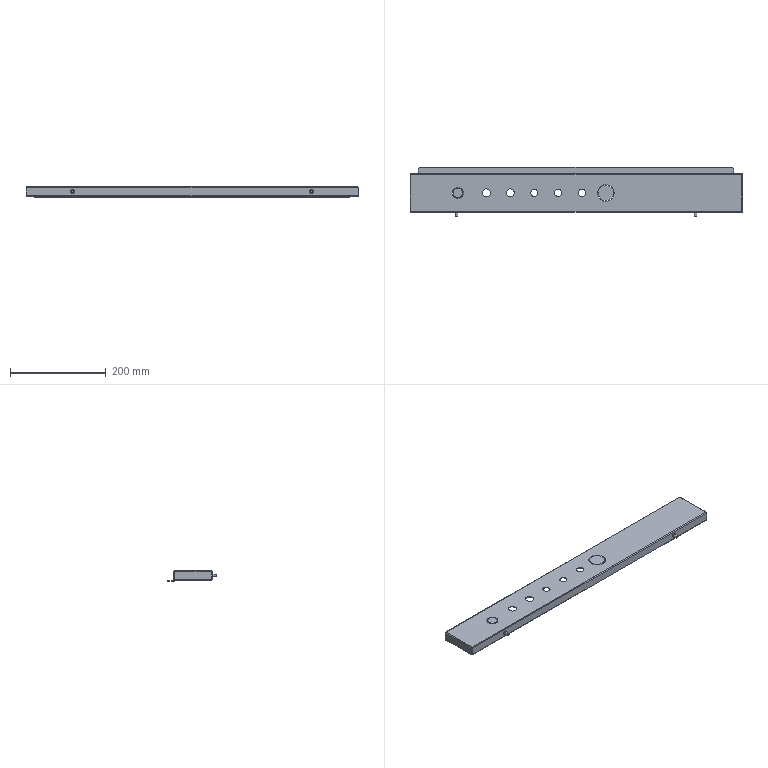Part | STEP file | FHD-021-003 rear door lower crossbeam | 1 solid | 145 faces | box 695 x 103 x 22 mm | volume 152226 mm3 | plane 81 | cylinder 51 | spline 13 | commonest cylinder face diameters 0.4 x8 3.4 x8 5.2 x4 20 x4 23 x4 32 x4